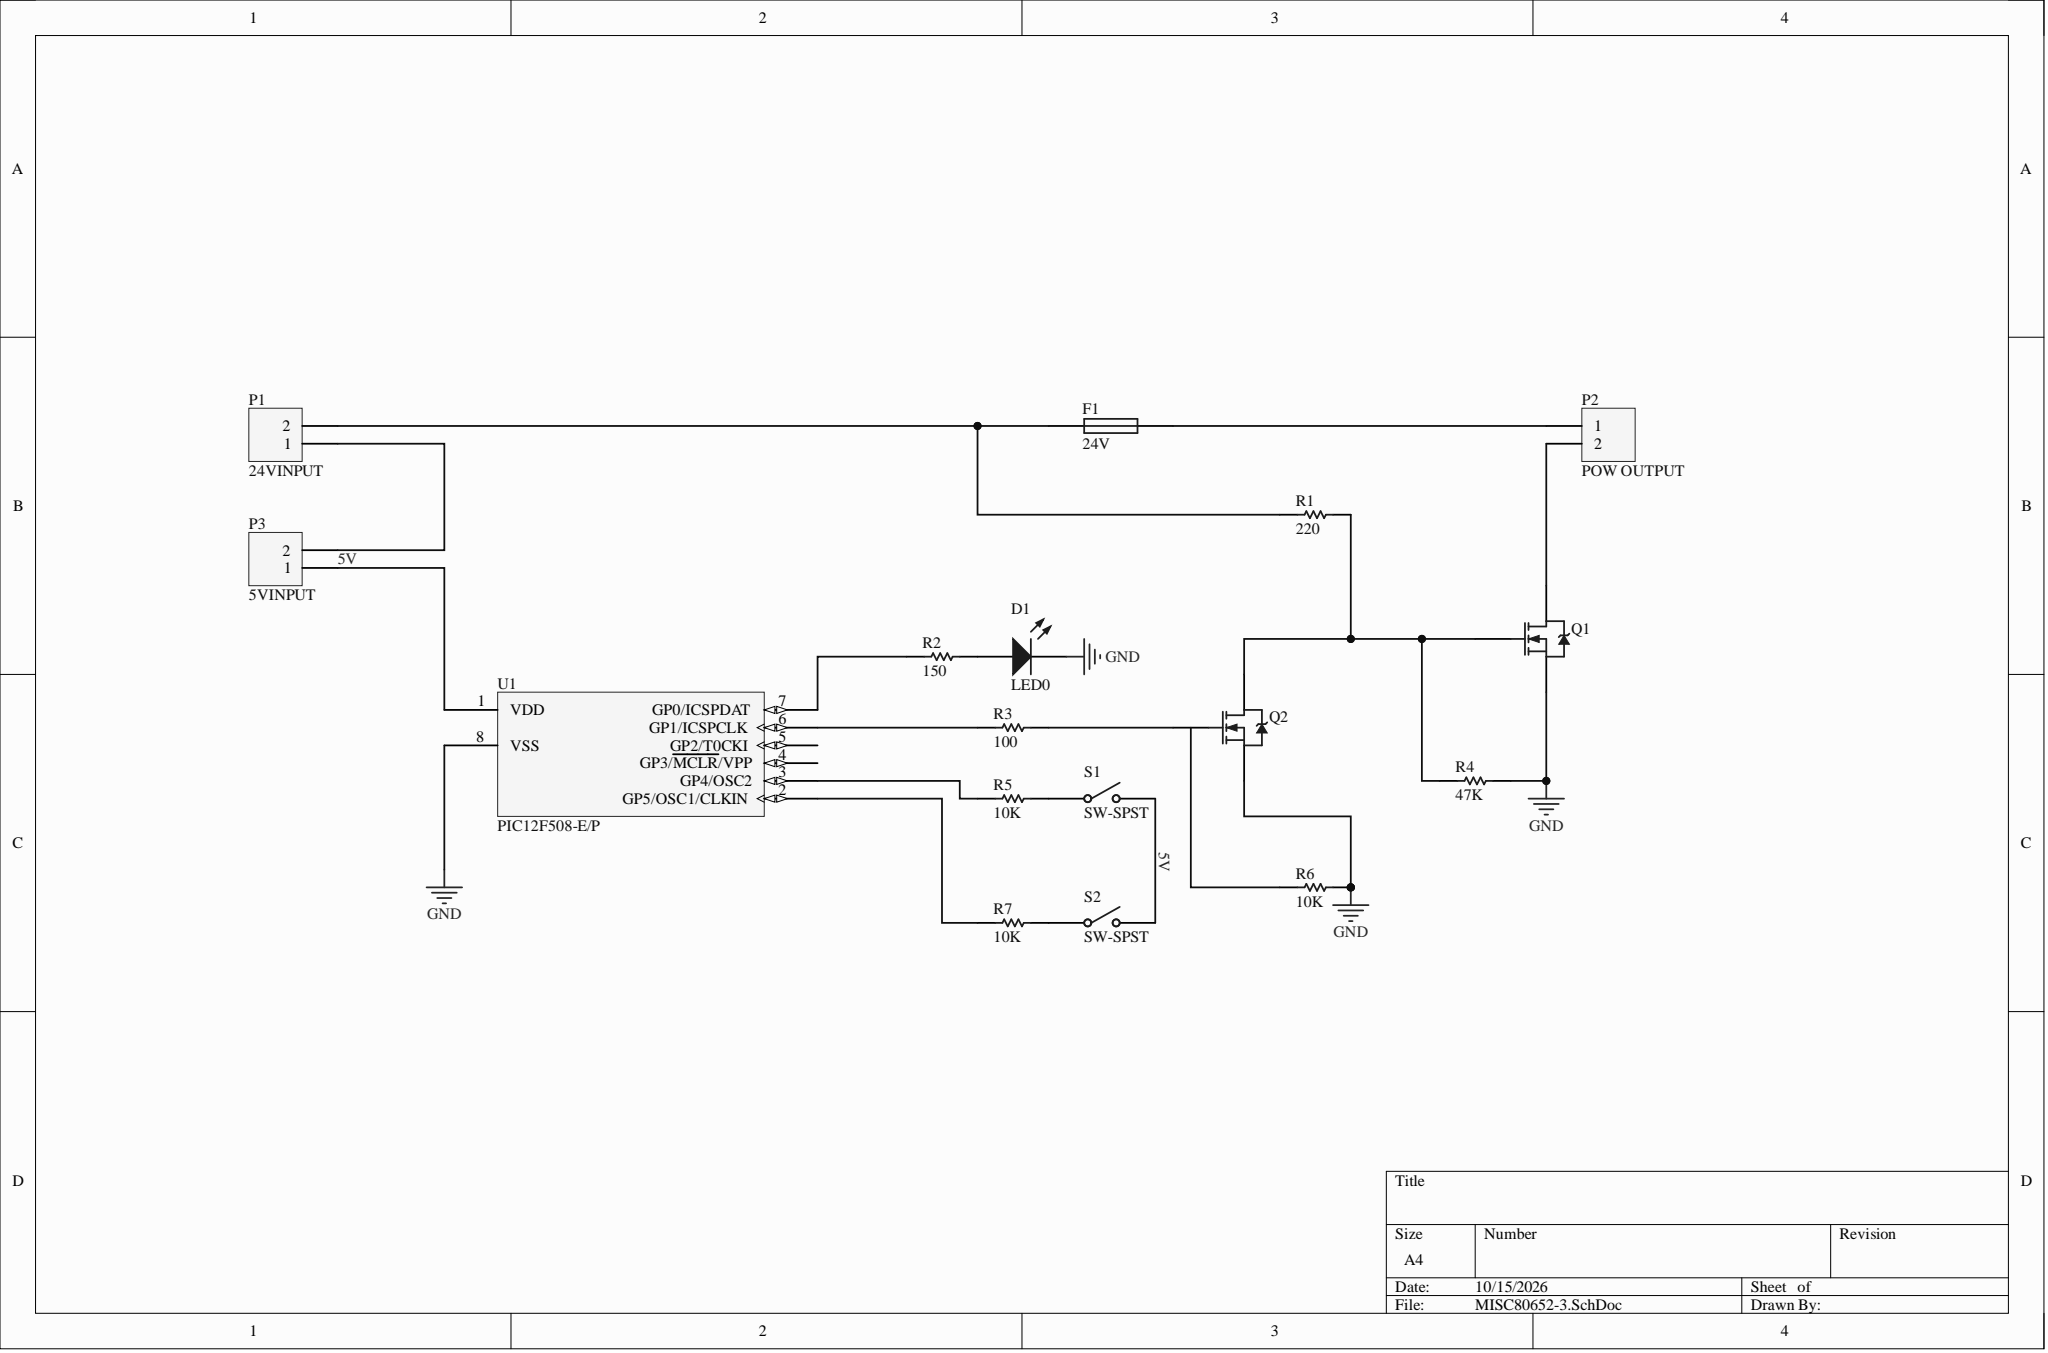Circuit board | Altium Designer | 17 parts | 15 nets
Bill of materials:
Comment,Description,Designator,Footprint,LibRef,Quantity
"LED0","Typical INFRARED GaAs LED","D1","LED-0","LED0","1"
"24V","Fuse","F1","PIN-W2/E2.8","Fuse 1","1"
"24VINPUT","Header, 2-Pin","P1","HDR1X2","Header 2","1"
"POW OUTPUT","Header, 2-Pin","P2","HDR1X2","Header 2","1"
"5VINPUT","Header, 2-Pin","P3","HDR1X2","Header 2","1"
"JANTXV2N7224","HEXFET Power MOSFET","Q1, Q2","TO-254AA","JANTXV2N7224","2"
"220","Resistor","R1","AXIAL-0.3","Res1","1"
"150","Resistor","R2","AXIAL-0.3","Res1","1"
"100","Resistor","R3","AXIAL-0.3","Res1","1"
"47K","Resistor","R4","AXIAL-0.3","Res1","1"
"10K","Resistor","R5, R6, R7","AXIAL-0.3","Res1","3"
"SW-SPST","Single-Pole, Single-Throw Switch","S1, S2","SPST-2","SW-SPST","2"
"PIC12F508-E/P","8-bit Flash Microcontroller, 512 (x12-Bit words) Program Memory, 25 Bytes Data Memory, 8-Pin PDIP, Extended Temperature","U1","PDIP300-P8","PIC12F508-E/P","1"
Netlist (Protel format):
[
D1
LED-0
LED0



]
[
F1
PIN-W2/E2.8
24V



]
[
P1
HDR1X2
24VINPUT



]
[
P2
HDR1X2
POW OUTPUT



]
[
P3
HDR1X2
5VINPUT



]
[
Q1
TO-254AA
JANTXV2N7224



]
[
Q2
TO-254AA
JANTXV2N7224



]
[
R1
AXIAL-0.3
220



]
[
R2
AXIAL-0.3
150



]
[
R3
AXIAL-0.3
100



]
[
R4
AXIAL-0.3
47K



]
[
R5
AXIAL-0.3
10K



]
[
R6
AXIAL-0.3
10K



]
[
R7
AXIAL-0.3
10K



]
[
S1
SPST-2
SW-SPST



]
[
S2
SPST-2
SW-SPST



]
[
U1
PDIP300-P8
PIC12F508-E/P



]
(
NetR7_2
R7-2
S2-1
)
(
NetR7_1
R7-1
U1-2
)
(
NetR5_2
R5-2
S1-1
)
(
NetR5_1
R5-1
U1-3
)
(
NetR3_1
R3-1
U1-6
)
(
NetR2_1
R2-1
U1-7
)
(
NetQ2_3
Q2-3
R3-2
)
(
NetQ1_3
Q1-3
Q2-1
R1-2
R4-1
)
(
NetP2_2
P2-2
Q1-1
)
(
NetP1_1
P1-1
P3-2
)
(
NetF1_2
F1-2
P2-1
)
(
NetF1_1
F1-1
P1-2
R1-1
)
(
NetD1_1
D1-1
R2-2
)
(
GND
D1-2
Q1-2
Q2-2
R4-2
R6-2
U1-8
)
(
5V
P3-1
S1-2
S2-2
U1-1
)